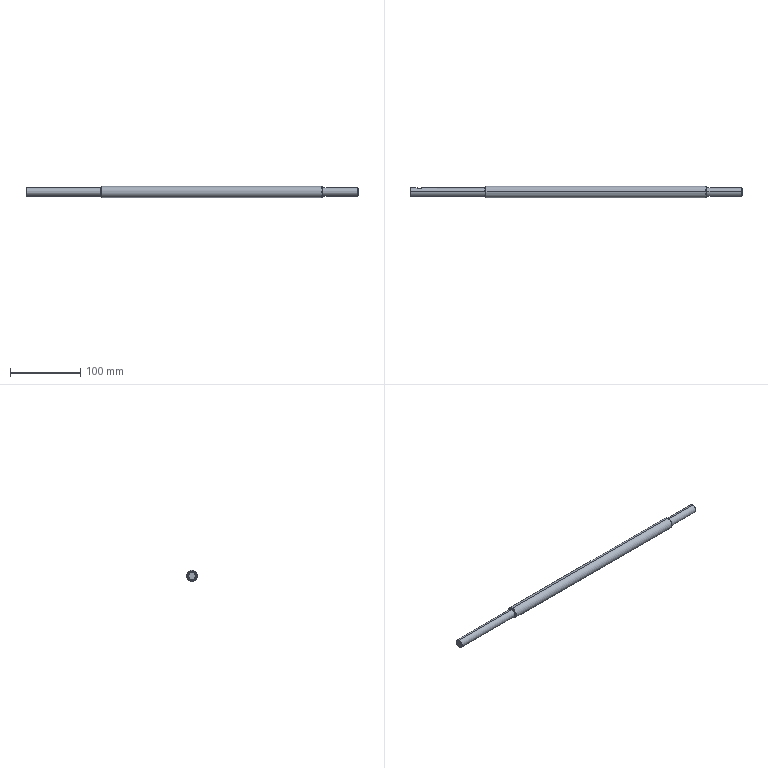Part | STEP file | 0232_001_MTSTR16-474 | 1 solid | 27 faces | box 474 x 16 x 16 mm | volume 81256 mm3 | plane 9 | cone 8 | cylinder 6 | spline 4 | commonest cylinder face diameters 12 x4 16 x2